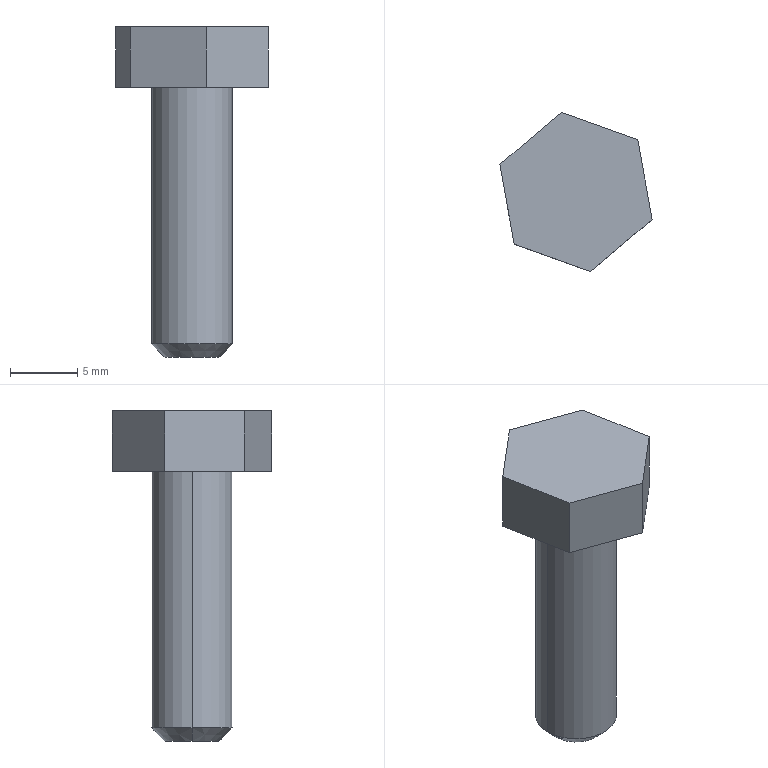Part | SolidWorks | features ICE 2, Chamfer 1, Extrusion 1 | 1 solid | 13 faces | box 11.292 x 11.809 x 24.5 mm | volume 977.997 mm3 | plane 9 | cone 2 | cylinder 2 | commonest cylinder face diameters 6 x2
STEP:
#1=CARTESIAN_POINT('',(-2.,0.,-20.));
#2=VERTEX_POINT('',#1);
#3=CARTESIAN_POINT('',(2.,0.,-20.));
#4=VERTEX_POINT('',#3);
#5=CARTESIAN_POINT('',(0.,0.,-20.));
#6=DIRECTION('',(0.,0.,-1.));
#7=DIRECTION('',(-1.,0.,0.));
#8=AXIS2_PLACEMENT_3D('',#5,#6,#7);
#9=CIRCLE('',#8,2.);
#10=EDGE_CURVE('',#2,#4,#9,.T.);
#11=ORIENTED_EDGE('',*,*,#10,.F.);
#12=CARTESIAN_POINT('',(-3.,0.,-19.));
#13=VERTEX_POINT('',#12);
#14=CARTESIAN_POINT('',(-2.,0.,-20.));
#15=DIRECTION('',(-0.7071,0.,0.7071));
#16=VECTOR('',#15,1000.);
#17=LINE('',#14,#16);
#18=EDGE_CURVE('',#2,#13,#17,.T.);
#19=ORIENTED_EDGE('',*,*,#18,.T.);
#20=CARTESIAN_POINT('',(3.,0.,-19.));
#21=VERTEX_POINT('',#20);
#22=CARTESIAN_POINT('',(0.,0.,-19.));
#23=DIRECTION('',(0.,0.,1.));
#24=DIRECTION('',(-1.,0.,0.));
#25=AXIS2_PLACEMENT_3D('',#22,#23,#24);
#26=CIRCLE('',#25,3.);
#27=EDGE_CURVE('',#21,#13,#26,.T.);
#28=ORIENTED_EDGE('',*,*,#27,.F.);
#29=CARTESIAN_POINT('',(2.,0.,-20.));
#30=DIRECTION('',(0.7071,0.,0.7071));
#31=VECTOR('',#30,1000.);
#32=LINE('',#29,#31);
#33=EDGE_CURVE('',#4,#21,#32,.T.);
#34=ORIENTED_EDGE('',*,*,#33,.F.);
#35=EDGE_LOOP('',(#11,#19,#28,#34));
#36=FACE_OUTER_BOUND('',#35,.T.);
#37=CARTESIAN_POINT('',(0.,0.,-20.));
#38=DIRECTION('',(0.,0.,1.));
#39=DIRECTION('',(1.,0.,0.));
#40=AXIS2_PLACEMENT_3D('',#37,#38,#39);
#41=CONICAL_SURFACE('',#40,2.,0.7854);
#42=ADVANCED_FACE('',(#36),#41,.T.);
#43=ORIENTED_EDGE('',*,*,#27,.T.);
#44=CARTESIAN_POINT('',(-3.,0.,0.));
#45=VERTEX_POINT('',#44);
#46=CARTESIAN_POINT('',(-3.,0.,-20.));
#47=DIRECTION('',(0.,0.,1.));
#48=VECTOR('',#47,1000.);
#49=LINE('',#46,#48);
#50=EDGE_CURVE('',#13,#45,#49,.T.);
#51=ORIENTED_EDGE('',*,*,#50,.T.);
#52=CARTESIAN_POINT('',(3.,0.,0.));
#53=VERTEX_POINT('',#52);
#54=CARTESIAN_POINT('',(0.,0.,0.));
#55=DIRECTION('',(0.,0.,-1.));
#56=DIRECTION('',(-1.,0.,0.));
#57=AXIS2_PLACEMENT_3D('',#54,#55,#56);
#58=CIRCLE('',#57,3.);
#59=EDGE_CURVE('',#45,#53,#58,.T.);
#60=ORIENTED_EDGE('',*,*,#59,.T.);
#61=CARTESIAN_POINT('',(3.,0.,-20.));
#62=DIRECTION('',(0.,0.,1.));
#63=VECTOR('',#62,1000.);
#64=LINE('',#61,#63);
#65=EDGE_CURVE('',#21,#53,#64,.T.);
#66=ORIENTED_EDGE('',*,*,#65,.F.);
#67=EDGE_LOOP('',(#43,#51,#60,#66));
#68=FACE_OUTER_BOUND('',#67,.T.);
#69=CARTESIAN_POINT('',(0.,0.,-20.));
#70=DIRECTION('',(0.,0.,1.));
#71=DIRECTION('',(1.,0.,0.));
#72=AXIS2_PLACEMENT_3D('',#69,#70,#71);
#73=CYLINDRICAL_SURFACE('',#72,3.);
#74=ADVANCED_FACE('',(#68),#73,.T.);
#75=CARTESIAN_POINT('',(0.,0.,0.));
#76=DIRECTION('',(0.,0.,-1.));
#77=DIRECTION('',(-1.,0.,0.));
#78=AXIS2_PLACEMENT_3D('',#75,#76,#77);
#79=CIRCLE('',#78,3.);
#80=EDGE_CURVE('',#53,#45,#79,.T.);
#81=ORIENTED_EDGE('',*,*,#80,.F.);
#82=ORIENTED_EDGE('',*,*,#59,.F.);
#83=EDGE_LOOP('',(#81,#82));
#84=FACE_BOUND('',#83,.T.);
#85=CARTESIAN_POINT('',(1.065,-5.905,0.));
#86=VERTEX_POINT('',#85);
#87=CARTESIAN_POINT('',(-4.581,-3.875,0.));
#88=VERTEX_POINT('',#87);
#89=CARTESIAN_POINT('',(1.065,-5.905,0.));
#90=DIRECTION('',(-0.941,0.3383,0.));
#91=VECTOR('',#90,1000.);
#92=LINE('',#89,#91);
#93=EDGE_CURVE('',#86,#88,#92,.T.);
#94=ORIENTED_EDGE('',*,*,#93,.T.);
#95=CARTESIAN_POINT('',(-5.646,2.03,0.));
#96=VERTEX_POINT('',#95);
#97=CARTESIAN_POINT('',(-4.581,-3.875,0.));
#98=DIRECTION('',(-0.1775,0.9841,0.));
#99=VECTOR('',#98,1000.);
#100=LINE('',#97,#99);
#101=EDGE_CURVE('',#88,#96,#100,.T.);
#102=ORIENTED_EDGE('',*,*,#101,.T.);
#103=CARTESIAN_POINT('',(-1.065,5.905,0.));
#104=VERTEX_POINT('',#103);
#105=CARTESIAN_POINT('',(-5.646,2.03,0.));
#106=DIRECTION('',(0.7635,0.6458,0.));
#107=VECTOR('',#106,1000.);
#108=LINE('',#105,#107);
#109=EDGE_CURVE('',#96,#104,#108,.T.);
#110=ORIENTED_EDGE('',*,*,#109,.T.);
#111=CARTESIAN_POINT('',(4.581,3.875,0.));
#112=VERTEX_POINT('',#111);
#113=CARTESIAN_POINT('',(-1.065,5.905,0.));
#114=DIRECTION('',(0.941,-0.3383,0.));
#115=VECTOR('',#114,1000.);
#116=LINE('',#113,#115);
#117=EDGE_CURVE('',#104,#112,#116,.T.);
#118=ORIENTED_EDGE('',*,*,#117,.T.);
#119=CARTESIAN_POINT('',(5.646,-2.03,0.));
#120=VERTEX_POINT('',#119);
#121=CARTESIAN_POINT('',(4.581,3.875,0.));
#122=DIRECTION('',(0.1775,-0.9841,0.));
#123=VECTOR('',#122,1000.);
#124=LINE('',#121,#123);
#125=EDGE_CURVE('',#112,#120,#124,.T.);
#126=ORIENTED_EDGE('',*,*,#125,.T.);
#127=CARTESIAN_POINT('',(5.646,-2.03,0.));
#128=DIRECTION('',(-0.7635,-0.6458,0.));
#129=VECTOR('',#128,1000.);
#130=LINE('',#127,#129);
#131=EDGE_CURVE('',#120,#86,#130,.T.);
#132=ORIENTED_EDGE('',*,*,#131,.T.);
#133=EDGE_LOOP('',(#94,#102,#110,#118,#126,#132));
#134=FACE_OUTER_BOUND('',#133,.T.);
#135=CARTESIAN_POINT('',(0.,0.,0.));
#136=DIRECTION('',(0.,0.,1.));
#137=DIRECTION('',(1.,0.,0.));
#138=AXIS2_PLACEMENT_3D('',#135,#136,#137);
#139=PLANE('',#138);
#140=ADVANCED_FACE('',(#84,#134),#139,.F.);
#141=ORIENTED_EDGE('',*,*,#93,.F.);
#142=CARTESIAN_POINT('',(1.065,-5.905,4.5));
#143=VERTEX_POINT('',#142);
#144=CARTESIAN_POINT('',(1.065,-5.905,4.5));
#145=DIRECTION('',(0.,0.,-1.));
#146=VECTOR('',#145,1000.);
#147=LINE('',#144,#146);
#148=EDGE_CURVE('',#143,#86,#147,.T.);
#149=ORIENTED_EDGE('',*,*,#148,.F.);
#150=CARTESIAN_POINT('',(-4.581,-3.875,4.5));
#151=VERTEX_POINT('',#150);
#152=CARTESIAN_POINT('',(1.065,-5.905,4.5));
#153=DIRECTION('',(-0.941,0.3383,0.));
#154=VECTOR('',#153,1000.);
#155=LINE('',#152,#154);
#156=EDGE_CURVE('',#143,#151,#155,.T.);
#157=ORIENTED_EDGE('',*,*,#156,.T.);
#158=CARTESIAN_POINT('',(-4.581,-3.875,4.5));
#159=DIRECTION('',(0.,0.,-1.));
#160=VECTOR('',#159,1000.);
#161=LINE('',#158,#160);
#162=EDGE_CURVE('',#151,#88,#161,.T.);
#163=ORIENTED_EDGE('',*,*,#162,.T.);
#164=EDGE_LOOP('',(#141,#149,#157,#163));
#165=FACE_OUTER_BOUND('',#164,.T.);
#166=CARTESIAN_POINT('',(1.065,-5.905,4.5));
#167=DIRECTION('',(-0.3383,-0.941,0.));
#168=DIRECTION('',(0.941,-0.3383,0.));
#169=AXIS2_PLACEMENT_3D('',#166,#167,#168);
#170=PLANE('',#169);
#171=ADVANCED_FACE('',(#165),#170,.T.);
#172=ORIENTED_EDGE('',*,*,#131,.F.);
#173=CARTESIAN_POINT('',(5.646,-2.03,4.5));
#174=VERTEX_POINT('',#173);
#175=CARTESIAN_POINT('',(5.646,-2.03,4.5));
#176=DIRECTION('',(0.,0.,-1.));
#177=VECTOR('',#176,1000.);
#178=LINE('',#175,#177);
#179=EDGE_CURVE('',#174,#120,#178,.T.);
#180=ORIENTED_EDGE('',*,*,#179,.F.);
#181=CARTESIAN_POINT('',(5.646,-2.03,4.5));
#182=DIRECTION('',(-0.7635,-0.6458,0.));
#183=VECTOR('',#182,1000.);
#184=LINE('',#181,#183);
#185=EDGE_CURVE('',#174,#143,#184,.T.);
#186=ORIENTED_EDGE('',*,*,#185,.T.);
#187=ORIENTED_EDGE('',*,*,#148,.T.);
#188=EDGE_LOOP('',(#172,#180,#186,#187));
#189=FACE_OUTER_BOUND('',#188,.T.);
#190=CARTESIAN_POINT('',(5.646,-2.03,4.5));
#191=DIRECTION('',(0.6458,-0.7635,0.));
#192=DIRECTION('',(0.7635,0.6458,0.));
#193=AXIS2_PLACEMENT_3D('',#190,#191,#192);
#194=PLANE('',#193);
#195=ADVANCED_FACE('',(#189),#194,.T.);
#196=ORIENTED_EDGE('',*,*,#125,.F.);
#197=CARTESIAN_POINT('',(4.581,3.875,4.5));
#198=VERTEX_POINT('',#197);
#199=CARTESIAN_POINT('',(4.581,3.875,4.5));
#200=DIRECTION('',(0.,0.,-1.));
#201=VECTOR('',#200,1000.);
#202=LINE('',#199,#201);
#203=EDGE_CURVE('',#198,#112,#202,.T.);
#204=ORIENTED_EDGE('',*,*,#203,.F.);
#205=CARTESIAN_POINT('',(4.581,3.875,4.5));
#206=DIRECTION('',(0.1775,-0.9841,0.));
#207=VECTOR('',#206,1000.);
#208=LINE('',#205,#207);
#209=EDGE_CURVE('',#198,#174,#208,.T.);
#210=ORIENTED_EDGE('',*,*,#209,.T.);
#211=ORIENTED_EDGE('',*,*,#179,.T.);
#212=EDGE_LOOP('',(#196,#204,#210,#211));
#213=FACE_OUTER_BOUND('',#212,.T.);
#214=CARTESIAN_POINT('',(4.581,3.875,4.5));
#215=DIRECTION('',(0.9841,0.1775,0.));
#216=DIRECTION('',(-0.1775,0.9841,0.));
#217=AXIS2_PLACEMENT_3D('',#214,#215,#216);
#218=PLANE('',#217);
#219=ADVANCED_FACE('',(#213),#218,.T.);
#220=ORIENTED_EDGE('',*,*,#117,.F.);
#221=CARTESIAN_POINT('',(-1.065,5.905,4.5));
#222=VERTEX_POINT('',#221);
#223=CARTESIAN_POINT('',(-1.065,5.905,4.5));
#224=DIRECTION('',(0.,0.,-1.));
#225=VECTOR('',#224,1000.);
#226=LINE('',#223,#225);
#227=EDGE_CURVE('',#222,#104,#226,.T.);
#228=ORIENTED_EDGE('',*,*,#227,.F.);
#229=CARTESIAN_POINT('',(-1.065,5.905,4.5));
#230=DIRECTION('',(0.941,-0.3383,0.));
#231=VECTOR('',#230,1000.);
#232=LINE('',#229,#231);
#233=EDGE_CURVE('',#222,#198,#232,.T.);
#234=ORIENTED_EDGE('',*,*,#233,.T.);
#235=ORIENTED_EDGE('',*,*,#203,.T.);
#236=EDGE_LOOP('',(#220,#228,#234,#235));
#237=FACE_OUTER_BOUND('',#236,.T.);
#238=CARTESIAN_POINT('',(-1.065,5.905,4.5));
#239=DIRECTION('',(0.3383,0.941,0.));
#240=DIRECTION('',(-0.941,0.3383,0.));
#241=AXIS2_PLACEMENT_3D('',#238,#239,#240);
#242=PLANE('',#241);
#243=ADVANCED_FACE('',(#237),#242,.T.);
#244=ORIENTED_EDGE('',*,*,#109,.F.);
#245=CARTESIAN_POINT('',(-5.646,2.03,4.5));
#246=VERTEX_POINT('',#245);
#247=CARTESIAN_POINT('',(-5.646,2.03,4.5));
#248=DIRECTION('',(0.,0.,-1.));
#249=VECTOR('',#248,1000.);
#250=LINE('',#247,#249);
#251=EDGE_CURVE('',#246,#96,#250,.T.);
#252=ORIENTED_EDGE('',*,*,#251,.F.);
#253=CARTESIAN_POINT('',(-5.646,2.03,4.5));
#254=DIRECTION('',(0.7635,0.6458,0.));
#255=VECTOR('',#254,1000.);
#256=LINE('',#253,#255);
#257=EDGE_CURVE('',#246,#222,#256,.T.);
#258=ORIENTED_EDGE('',*,*,#257,.T.);
#259=ORIENTED_EDGE('',*,*,#227,.T.);
#260=EDGE_LOOP('',(#244,#252,#258,#259));
#261=FACE_OUTER_BOUND('',#260,.T.);
#262=CARTESIAN_POINT('',(-5.646,2.03,4.5));
#263=DIRECTION('',(-0.6458,0.7635,0.));
#264=DIRECTION('',(-0.7635,-0.6458,0.));
#265=AXIS2_PLACEMENT_3D('',#262,#263,#264);
#266=PLANE('',#265);
#267=ADVANCED_FACE('',(#261),#266,.T.);
#268=ORIENTED_EDGE('',*,*,#101,.F.);
#269=ORIENTED_EDGE('',*,*,#162,.F.);
#270=CARTESIAN_POINT('',(-4.581,-3.875,4.5));
#271=DIRECTION('',(-0.1775,0.9841,0.));
#272=VECTOR('',#271,1000.);
#273=LINE('',#270,#272);
#274=EDGE_CURVE('',#151,#246,#273,.T.);
#275=ORIENTED_EDGE('',*,*,#274,.T.);
#276=ORIENTED_EDGE('',*,*,#251,.T.);
#277=EDGE_LOOP('',(#268,#269,#275,#276));
#278=FACE_OUTER_BOUND('',#277,.T.);
#279=CARTESIAN_POINT('',(-4.581,-3.875,4.5));
#280=DIRECTION('',(-0.9841,-0.1775,0.));
#281=DIRECTION('',(0.1775,-0.9841,0.));
#282=AXIS2_PLACEMENT_3D('',#279,#280,#281);
#283=PLANE('',#282);
#284=ADVANCED_FACE('',(#278),#283,.T.);
#285=ORIENTED_EDGE('',*,*,#274,.F.);
#286=ORIENTED_EDGE('',*,*,#156,.F.);
#287=ORIENTED_EDGE('',*,*,#185,.F.);
#288=ORIENTED_EDGE('',*,*,#209,.F.);
#289=ORIENTED_EDGE('',*,*,#233,.F.);
#290=ORIENTED_EDGE('',*,*,#257,.F.);
#291=EDGE_LOOP('',(#285,#286,#287,#288,#289,#290));
#292=FACE_OUTER_BOUND('',#291,.T.);
#293=CARTESIAN_POINT('',(0.,0.,4.5));
#294=DIRECTION('',(0.,0.,1.));
#295=DIRECTION('',(1.,0.,0.));
#296=AXIS2_PLACEMENT_3D('',#293,#294,#295);
#297=PLANE('',#296);
#298=ADVANCED_FACE('',(#292),#297,.T.);
#299=ORIENTED_EDGE('',*,*,#50,.F.);
#300=CARTESIAN_POINT('',(0.,0.,-19.));
#301=DIRECTION('',(0.,0.,1.));
#302=DIRECTION('',(-1.,0.,0.));
#303=AXIS2_PLACEMENT_3D('',#300,#301,#302);
#304=CIRCLE('',#303,3.);
#305=EDGE_CURVE('',#13,#21,#304,.T.);
#306=ORIENTED_EDGE('',*,*,#305,.T.);
#307=ORIENTED_EDGE('',*,*,#65,.T.);
#308=ORIENTED_EDGE('',*,*,#80,.T.);
#309=EDGE_LOOP('',(#299,#306,#307,#308));
#310=FACE_OUTER_BOUND('',#309,.T.);
#311=CARTESIAN_POINT('',(0.,0.,-20.));
#312=DIRECTION('',(0.,0.,1.));
#313=DIRECTION('',(1.,0.,0.));
#314=AXIS2_PLACEMENT_3D('',#311,#312,#313);
#315=CYLINDRICAL_SURFACE('',#314,3.);
#316=ADVANCED_FACE('',(#310),#315,.T.);
#317=CARTESIAN_POINT('',(0.,0.,-20.));
#318=DIRECTION('',(0.,0.,-1.));
#319=DIRECTION('',(-1.,0.,0.));
#320=AXIS2_PLACEMENT_3D('',#317,#318,#319);
#321=CIRCLE('',#320,2.);
#322=EDGE_CURVE('',#4,#2,#321,.T.);
#323=ORIENTED_EDGE('',*,*,#322,.T.);
#324=ORIENTED_EDGE('',*,*,#10,.T.);
#325=EDGE_LOOP('',(#323,#324));
#326=FACE_OUTER_BOUND('',#325,.T.);
#327=CARTESIAN_POINT('',(0.,0.,-20.));
#328=DIRECTION('',(0.,0.,-1.));
#329=DIRECTION('',(-1.,0.,0.));
#330=AXIS2_PLACEMENT_3D('',#327,#328,#329);
#331=PLANE('',#330);
#332=ADVANCED_FACE('',(#326),#331,.T.);
#333=ORIENTED_EDGE('',*,*,#18,.F.);
#334=ORIENTED_EDGE('',*,*,#322,.F.);
#335=ORIENTED_EDGE('',*,*,#33,.T.);
#336=ORIENTED_EDGE('',*,*,#305,.F.);
#337=EDGE_LOOP('',(#333,#334,#335,#336));
#338=FACE_OUTER_BOUND('',#337,.T.);
#339=CARTESIAN_POINT('',(0.,0.,-20.));
#340=DIRECTION('',(0.,0.,1.));
#341=DIRECTION('',(1.,0.,0.));
#342=AXIS2_PLACEMENT_3D('',#339,#340,#341);
#343=CONICAL_SURFACE('',#342,2.,0.7854);
#344=ADVANCED_FACE('',(#338),#343,.T.);
#345=CLOSED_SHELL('',(#42,#74,#140,#171,#195,#219,#243,#267,#284,#298,#316,#332,#344));
#346=MANIFOLD_SOLID_BREP('',#345);
#347=CARTESIAN_POINT('',(0.,0.,0.));
#348=DIRECTION('',(0.,0.,1.));
#349=DIRECTION('',(1.,0.,0.));
#350=AXIS2_PLACEMENT_3D('',#347,#348,#349);
#351=(LENGTH_UNIT()NAMED_UNIT(*)SI_UNIT(.MILLI.,.METRE.));
#352=UNCERTAINTY_MEASURE_WITH_UNIT(LENGTH_MEASURE(0.00001),#351,'','');
#353=(NAMED_UNIT(*)PLANE_ANGLE_UNIT()SI_UNIT($,.RADIAN.));
#354=(NAMED_UNIT(*)SI_UNIT($,.STERADIAN.)SOLID_ANGLE_UNIT());
#355=(GEOMETRIC_REPRESENTATION_CONTEXT(3)GLOBAL_UNCERTAINTY_ASSIGNED_CONTEXT((#352))GLOBAL_UNIT_ASSIGNED_CONTEXT((#351,#353,#354))REPRESENTATION_CONTEXT('',''));
#356=ADVANCED_BREP_SHAPE_REPRESENTATION('',(#346,#350),#355);